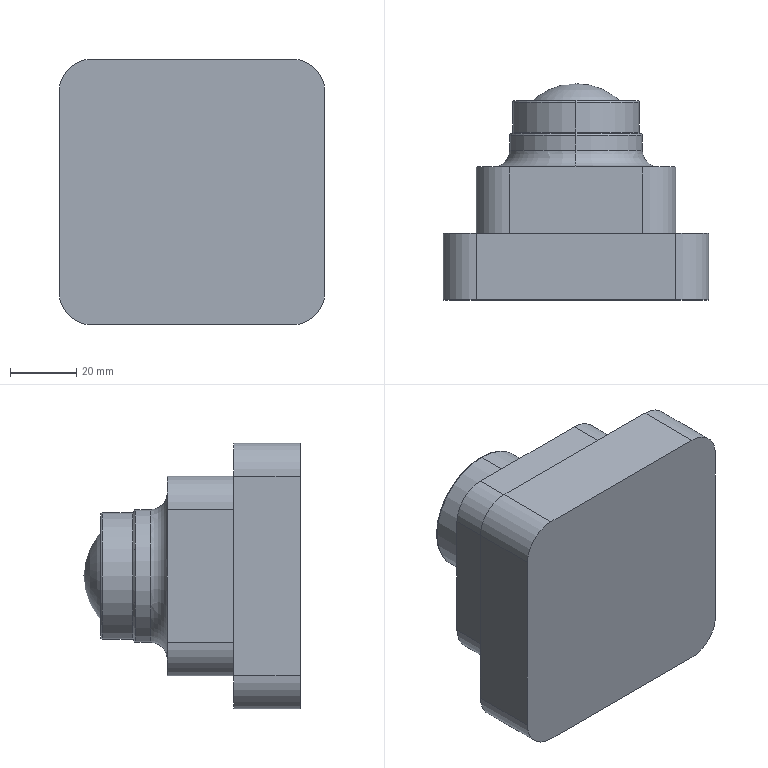Part | SolidWorks | features ICE 5, Fillet 2, Dome 1, Extrusion 1 | 1 solid | 40 faces | box 80 x 65.1 x 80 mm | volume 221973 mm3 | cylinder 16 | plane 13 | torus 10 | sphere 1 | commonest cylinder face diameters 20 x8 30 x2 35 x2 38 x2 40 x2
STEP:
#1=CARTESIAN_POINT('',(0.,49.5,-20.));
#2=VERTEX_POINT('',#1);
#3=CARTESIAN_POINT('',(0.,49.5,20.));
#4=VERTEX_POINT('',#3);
#5=CARTESIAN_POINT('',(0.,49.5,0.));
#6=DIRECTION('',(0.,-1.,0.));
#7=DIRECTION('',(0.,0.,1.));
#8=AXIS2_PLACEMENT_3D('',#5,#6,#7);
#9=CIRCLE('',#8,20.);
#10=EDGE_CURVE('',#2,#4,#9,.T.);
#11=ORIENTED_EDGE('',*,*,#10,.F.);
#12=CARTESIAN_POINT('',(0.,50.,-19.5));
#13=VERTEX_POINT('',#12);
#14=CARTESIAN_POINT('',(0.,49.5,-19.5));
#15=DIRECTION('',(1.,0.,0.));
#16=DIRECTION('',(0.,0.,-1.));
#17=AXIS2_PLACEMENT_3D('',#14,#15,#16);
#18=CIRCLE('',#17,0.5);
#19=EDGE_CURVE('',#2,#13,#18,.T.);
#20=ORIENTED_EDGE('',*,*,#19,.T.);
#21=CARTESIAN_POINT('',(0.,50.,19.5));
#22=VERTEX_POINT('',#21);
#23=CARTESIAN_POINT('',(0.,50.,0.));
#24=DIRECTION('',(0.,-1.,0.));
#25=DIRECTION('',(0.,0.,1.));
#26=AXIS2_PLACEMENT_3D('',#23,#24,#25);
#27=CIRCLE('',#26,19.5);
#28=EDGE_CURVE('',#13,#22,#27,.T.);
#29=ORIENTED_EDGE('',*,*,#28,.T.);
#30=CARTESIAN_POINT('',(0.,49.5,19.5));
#31=DIRECTION('',(-1.,0.,0.));
#32=DIRECTION('',(0.,0.,1.));
#33=AXIS2_PLACEMENT_3D('',#30,#31,#32);
#34=CIRCLE('',#33,0.5);
#35=EDGE_CURVE('',#4,#22,#34,.T.);
#36=ORIENTED_EDGE('',*,*,#35,.F.);
#37=EDGE_LOOP('',(#11,#20,#29,#36));
#38=FACE_OUTER_BOUND('',#37,.T.);
#39=CARTESIAN_POINT('',(0.,49.5,0.));
#40=DIRECTION('',(0.,1.,0.));
#41=DIRECTION('',(0.,0.,1.));
#42=AXIS2_PLACEMENT_3D('',#39,#40,#41);
#43=TOROIDAL_SURFACE('',#42,19.5,0.5);
#44=ADVANCED_FACE('',(#38),#43,.T.);
#45=CARTESIAN_POINT('',(0.,50.5,-19.));
#46=VERTEX_POINT('',#45);
#47=CARTESIAN_POINT('',(0.,50.5,19.));
#48=VERTEX_POINT('',#47);
#49=CARTESIAN_POINT('',(0.,50.5,0.));
#50=DIRECTION('',(0.,1.,0.));
#51=DIRECTION('',(0.,0.,1.));
#52=AXIS2_PLACEMENT_3D('',#49,#50,#51);
#53=CIRCLE('',#52,19.);
#54=EDGE_CURVE('',#46,#48,#53,.T.);
#55=ORIENTED_EDGE('',*,*,#54,.F.);
#56=CARTESIAN_POINT('',(0.,50.5,-19.5));
#57=DIRECTION('',(1.,0.,0.));
#58=DIRECTION('',(0.,0.,-1.));
#59=AXIS2_PLACEMENT_3D('',#56,#57,#58);
#60=CIRCLE('',#59,0.5);
#61=EDGE_CURVE('',#46,#13,#60,.T.);
#62=ORIENTED_EDGE('',*,*,#61,.T.);
#63=CARTESIAN_POINT('',(0.,50.,0.));
#64=DIRECTION('',(0.,-1.,0.));
#65=DIRECTION('',(0.,0.,1.));
#66=AXIS2_PLACEMENT_3D('',#63,#64,#65);
#67=CIRCLE('',#66,19.5);
#68=EDGE_CURVE('',#22,#13,#67,.T.);
#69=ORIENTED_EDGE('',*,*,#68,.F.);
#70=CARTESIAN_POINT('',(0.,50.5,19.5));
#71=DIRECTION('',(-1.,0.,0.));
#72=DIRECTION('',(0.,0.,1.));
#73=AXIS2_PLACEMENT_3D('',#70,#71,#72);
#74=CIRCLE('',#73,0.5);
#75=EDGE_CURVE('',#48,#22,#74,.T.);
#76=ORIENTED_EDGE('',*,*,#75,.F.);
#77=EDGE_LOOP('',(#55,#62,#69,#76));
#78=FACE_OUTER_BOUND('',#77,.T.);
#79=CARTESIAN_POINT('',(0.,50.5,0.));
#80=DIRECTION('',(0.,1.,0.));
#81=DIRECTION('',(0.,0.,1.));
#82=AXIS2_PLACEMENT_3D('',#79,#80,#81);
#83=TOROIDAL_SURFACE('',#82,19.5,0.5);
#84=ADVANCED_FACE('',(#78),#83,.F.);
#85=CARTESIAN_POINT('',(0.,59.5,-19.));
#86=VERTEX_POINT('',#85);
#87=CARTESIAN_POINT('',(0.,59.5,19.));
#88=VERTEX_POINT('',#87);
#89=CARTESIAN_POINT('',(0.,59.5,0.));
#90=DIRECTION('',(0.,-1.,0.));
#91=DIRECTION('',(0.,0.,1.));
#92=AXIS2_PLACEMENT_3D('',#89,#90,#91);
#93=CIRCLE('',#92,19.);
#94=EDGE_CURVE('',#86,#88,#93,.T.);
#95=ORIENTED_EDGE('',*,*,#94,.F.);
#96=CARTESIAN_POINT('',(0.,60.,-18.5));
#97=VERTEX_POINT('',#96);
#98=CARTESIAN_POINT('',(0.,59.5,-18.5));
#99=DIRECTION('',(1.,0.,0.));
#100=DIRECTION('',(0.,0.,-1.));
#101=AXIS2_PLACEMENT_3D('',#98,#99,#100);
#102=CIRCLE('',#101,0.5);
#103=EDGE_CURVE('',#86,#97,#102,.T.);
#104=ORIENTED_EDGE('',*,*,#103,.T.);
#105=CARTESIAN_POINT('',(0.,60.,18.5));
#106=VERTEX_POINT('',#105);
#107=CARTESIAN_POINT('',(0.,60.,0.));
#108=DIRECTION('',(0.,1.,0.));
#109=DIRECTION('',(0.,0.,1.));
#110=AXIS2_PLACEMENT_3D('',#107,#108,#109);
#111=CIRCLE('',#110,18.5);
#112=EDGE_CURVE('',#106,#97,#111,.T.);
#113=ORIENTED_EDGE('',*,*,#112,.F.);
#114=CARTESIAN_POINT('',(0.,59.5,18.5));
#115=DIRECTION('',(-1.,0.,0.));
#116=DIRECTION('',(0.,0.,1.));
#117=AXIS2_PLACEMENT_3D('',#114,#115,#116);
#118=CIRCLE('',#117,0.5);
#119=EDGE_CURVE('',#88,#106,#118,.T.);
#120=ORIENTED_EDGE('',*,*,#119,.F.);
#121=EDGE_LOOP('',(#95,#104,#113,#120));
#122=FACE_OUTER_BOUND('',#121,.T.);
#123=CARTESIAN_POINT('',(0.,59.5,0.));
#124=DIRECTION('',(0.,1.,0.));
#125=DIRECTION('',(0.,0.,1.));
#126=AXIS2_PLACEMENT_3D('',#123,#124,#125);
#127=TOROIDAL_SURFACE('',#126,18.5,0.5);
#128=ADVANCED_FACE('',(#122),#127,.T.);
#129=CARTESIAN_POINT('',(0.,60.,-18.));
#130=VERTEX_POINT('',#129);
#131=CARTESIAN_POINT('',(0.,60.,18.));
#132=VERTEX_POINT('',#131);
#133=CARTESIAN_POINT('',(0.,60.,0.));
#134=DIRECTION('',(0.,-1.,0.));
#135=DIRECTION('',(0.,0.,1.));
#136=AXIS2_PLACEMENT_3D('',#133,#134,#135);
#137=CIRCLE('',#136,18.);
#138=EDGE_CURVE('',#130,#132,#137,.T.);
#139=ORIENTED_EDGE('',*,*,#138,.F.);
#140=CARTESIAN_POINT('',(0.,59.5,-17.5));
#141=VERTEX_POINT('',#140);
#142=CARTESIAN_POINT('',(0.,59.5,-18.));
#143=DIRECTION('',(1.,0.,0.));
#144=DIRECTION('',(0.,0.,-1.));
#145=AXIS2_PLACEMENT_3D('',#142,#143,#144);
#146=CIRCLE('',#145,0.5);
#147=EDGE_CURVE('',#130,#141,#146,.T.);
#148=ORIENTED_EDGE('',*,*,#147,.T.);
#149=CARTESIAN_POINT('',(0.,59.5,17.5));
#150=VERTEX_POINT('',#149);
#151=CARTESIAN_POINT('',(0.,59.5,0.));
#152=DIRECTION('',(0.,1.,0.));
#153=DIRECTION('',(0.,0.,1.));
#154=AXIS2_PLACEMENT_3D('',#151,#152,#153);
#155=CIRCLE('',#154,17.5);
#156=EDGE_CURVE('',#150,#141,#155,.T.);
#157=ORIENTED_EDGE('',*,*,#156,.F.);
#158=CARTESIAN_POINT('',(0.,59.5,18.));
#159=DIRECTION('',(-1.,0.,0.));
#160=DIRECTION('',(0.,0.,1.));
#161=AXIS2_PLACEMENT_3D('',#158,#159,#160);
#162=CIRCLE('',#161,0.5);
#163=EDGE_CURVE('',#132,#150,#162,.T.);
#164=ORIENTED_EDGE('',*,*,#163,.F.);
#165=EDGE_LOOP('',(#139,#148,#157,#164));
#166=FACE_OUTER_BOUND('',#165,.T.);
#167=CARTESIAN_POINT('',(0.,59.5,0.));
#168=DIRECTION('',(0.,1.,0.));
#169=DIRECTION('',(0.,0.,1.));
#170=AXIS2_PLACEMENT_3D('',#167,#168,#169);
#171=TOROIDAL_SURFACE('',#170,18.,0.5);
#172=ADVANCED_FACE('',(#166),#171,.T.);
#173=CARTESIAN_POINT('',(0.,40.,25.));
#174=VERTEX_POINT('',#173);
#175=CARTESIAN_POINT('',(0.,40.,-25.));
#176=VERTEX_POINT('',#175);
#177=CARTESIAN_POINT('',(0.,40.,0.));
#178=DIRECTION('',(0.,-1.,0.));
#179=DIRECTION('',(0.,0.,-1.));
#180=AXIS2_PLACEMENT_3D('',#177,#178,#179);
#181=CIRCLE('',#180,25.);
#182=EDGE_CURVE('',#174,#176,#181,.T.);
#183=ORIENTED_EDGE('',*,*,#182,.F.);
#184=CARTESIAN_POINT('',(0.,45.,20.));
#185=VERTEX_POINT('',#184);
#186=CARTESIAN_POINT('',(0.,45.,25.));
#187=DIRECTION('',(1.,0.,0.));
#188=DIRECTION('',(0.,0.,-1.));
#189=AXIS2_PLACEMENT_3D('',#186,#187,#188);
#190=CIRCLE('',#189,5.);
#191=EDGE_CURVE('',#174,#185,#190,.T.);
#192=ORIENTED_EDGE('',*,*,#191,.T.);
#193=CARTESIAN_POINT('',(0.,45.,-20.));
#194=VERTEX_POINT('',#193);
#195=CARTESIAN_POINT('',(0.,45.,0.));
#196=DIRECTION('',(0.,1.,0.));
#197=DIRECTION('',(0.,0.,-1.));
#198=AXIS2_PLACEMENT_3D('',#195,#196,#197);
#199=CIRCLE('',#198,20.);
#200=EDGE_CURVE('',#194,#185,#199,.T.);
#201=ORIENTED_EDGE('',*,*,#200,.F.);
#202=CARTESIAN_POINT('',(0.,45.,-25.));
#203=DIRECTION('',(-1.,0.,0.));
#204=DIRECTION('',(0.,0.,1.));
#205=AXIS2_PLACEMENT_3D('',#202,#203,#204);
#206=CIRCLE('',#205,5.);
#207=EDGE_CURVE('',#176,#194,#206,.T.);
#208=ORIENTED_EDGE('',*,*,#207,.F.);
#209=EDGE_LOOP('',(#183,#192,#201,#208));
#210=FACE_OUTER_BOUND('',#209,.T.);
#211=CARTESIAN_POINT('',(0.,45.,0.));
#212=DIRECTION('',(0.,-1.,0.));
#213=DIRECTION('',(0.,0.,-1.));
#214=AXIS2_PLACEMENT_3D('',#211,#212,#213);
#215=TOROIDAL_SURFACE('',#214,25.,5.);
#216=ADVANCED_FACE('',(#210),#215,.F.);
#217=CARTESIAN_POINT('',(0.,58.1,15.));
#218=VERTEX_POINT('',#217);
#219=CARTESIAN_POINT('',(0.,58.1,-15.));
#220=VERTEX_POINT('',#219);
#221=CARTESIAN_POINT('',(0.,58.1,0.));
#222=DIRECTION('',(0.,1.,0.));
#223=DIRECTION('',(0.,0.,1.));
#224=AXIS2_PLACEMENT_3D('',#221,#222,#223);
#225=CIRCLE('',#224,15.);
#226=EDGE_CURVE('',#218,#220,#225,.T.);
#227=ORIENTED_EDGE('',*,*,#226,.F.);
#228=CARTESIAN_POINT('',(0.,58.,15.));
#229=VERTEX_POINT('',#228);
#230=CARTESIAN_POINT('',(0.,58.1,15.));
#231=DIRECTION('',(0.,-1.,0.));
#232=VECTOR('',#231,1000.);
#233=LINE('',#230,#232);
#234=EDGE_CURVE('',#218,#229,#233,.T.);
#235=ORIENTED_EDGE('',*,*,#234,.T.);
#236=CARTESIAN_POINT('',(0.,58.,-15.));
#237=VERTEX_POINT('',#236);
#238=CARTESIAN_POINT('',(0.,58.,0.));
#239=DIRECTION('',(0.,1.,0.));
#240=DIRECTION('',(0.,0.,1.));
#241=AXIS2_PLACEMENT_3D('',#238,#239,#240);
#242=CIRCLE('',#241,15.);
#243=EDGE_CURVE('',#229,#237,#242,.T.);
#244=ORIENTED_EDGE('',*,*,#243,.T.);
#245=CARTESIAN_POINT('',(0.,58.1,-15.));
#246=DIRECTION('',(0.,-1.,0.));
#247=VECTOR('',#246,1000.);
#248=LINE('',#245,#247);
#249=EDGE_CURVE('',#220,#237,#248,.T.);
#250=ORIENTED_EDGE('',*,*,#249,.F.);
#251=EDGE_LOOP('',(#227,#235,#244,#250));
#252=FACE_OUTER_BOUND('',#251,.T.);
#253=CARTESIAN_POINT('',(0.,58.1,0.));
#254=DIRECTION('',(0.,-1.,0.));
#255=DIRECTION('',(0.,0.,-1.));
#256=AXIS2_PLACEMENT_3D('',#253,#254,#255);
#257=CYLINDRICAL_SURFACE('',#256,15.);
#258=ADVANCED_FACE('',(#252),#257,.T.);
#259=CARTESIAN_POINT('',(0.,58.,-17.5));
#260=VERTEX_POINT('',#259);
#261=CARTESIAN_POINT('',(0.,58.,17.5));
#262=VERTEX_POINT('',#261);
#263=CARTESIAN_POINT('',(0.,58.,0.));
#264=DIRECTION('',(0.,1.,0.));
#265=DIRECTION('',(0.,0.,1.));
#266=AXIS2_PLACEMENT_3D('',#263,#264,#265);
#267=CIRCLE('',#266,17.5);
#268=EDGE_CURVE('',#260,#262,#267,.T.);
#269=ORIENTED_EDGE('',*,*,#268,.F.);
#270=CARTESIAN_POINT('',(0.,58.,-17.5));
#271=DIRECTION('',(0.,1.,0.));
#272=VECTOR('',#271,1000.);
#273=LINE('',#270,#272);
#274=EDGE_CURVE('',#260,#141,#273,.T.);
#275=ORIENTED_EDGE('',*,*,#274,.T.);
#276=CARTESIAN_POINT('',(0.,59.5,0.));
#277=DIRECTION('',(0.,1.,0.));
#278=DIRECTION('',(0.,0.,1.));
#279=AXIS2_PLACEMENT_3D('',#276,#277,#278);
#280=CIRCLE('',#279,17.5);
#281=EDGE_CURVE('',#141,#150,#280,.T.);
#282=ORIENTED_EDGE('',*,*,#281,.T.);
#283=CARTESIAN_POINT('',(0.,58.,17.5));
#284=DIRECTION('',(0.,1.,0.));
#285=VECTOR('',#284,1000.);
#286=LINE('',#283,#285);
#287=EDGE_CURVE('',#262,#150,#286,.T.);
#288=ORIENTED_EDGE('',*,*,#287,.F.);
#289=EDGE_LOOP('',(#269,#275,#282,#288));
#290=FACE_OUTER_BOUND('',#289,.T.);
#291=CARTESIAN_POINT('',(0.,58.,0.));
#292=DIRECTION('',(0.,1.,0.));
#293=DIRECTION('',(0.,0.,1.));
#294=AXIS2_PLACEMENT_3D('',#291,#292,#293);
#295=CYLINDRICAL_SURFACE('',#294,17.5);
#296=ADVANCED_FACE('',(#290),#295,.F.);
#297=ORIENTED_EDGE('',*,*,#94,.T.);
#298=CARTESIAN_POINT('',(0.,60.,19.));
#299=DIRECTION('',(0.,-1.,0.));
#300=VECTOR('',#299,1000.);
#301=LINE('',#298,#300);
#302=EDGE_CURVE('',#88,#48,#301,.T.);
#303=ORIENTED_EDGE('',*,*,#302,.T.);
#304=CARTESIAN_POINT('',(0.,50.5,0.));
#305=DIRECTION('',(0.,1.,0.));
#306=DIRECTION('',(0.,0.,1.));
#307=AXIS2_PLACEMENT_3D('',#304,#305,#306);
#308=CIRCLE('',#307,19.);
#309=EDGE_CURVE('',#48,#46,#308,.T.);
#310=ORIENTED_EDGE('',*,*,#309,.T.);
#311=CARTESIAN_POINT('',(0.,60.,-19.));
#312=DIRECTION('',(0.,-1.,0.));
#313=VECTOR('',#312,1000.);
#314=LINE('',#311,#313);
#315=EDGE_CURVE('',#86,#46,#314,.T.);
#316=ORIENTED_EDGE('',*,*,#315,.F.);
#317=EDGE_LOOP('',(#297,#303,#310,#316));
#318=FACE_OUTER_BOUND('',#317,.T.);
#319=CARTESIAN_POINT('',(0.,60.,0.));
#320=DIRECTION('',(0.,-1.,0.));
#321=DIRECTION('',(0.,0.,-1.));
#322=AXIS2_PLACEMENT_3D('',#319,#320,#321);
#323=CYLINDRICAL_SURFACE('',#322,19.);
#324=ADVANCED_FACE('',(#318),#323,.T.);
#325=ORIENTED_EDGE('',*,*,#10,.T.);
#326=CARTESIAN_POINT('',(0.,50.,20.));
#327=DIRECTION('',(0.,-1.,0.));
#328=VECTOR('',#327,1000.);
#329=LINE('',#326,#328);
#330=EDGE_CURVE('',#4,#185,#329,.T.);
#331=ORIENTED_EDGE('',*,*,#330,.T.);
#332=CARTESIAN_POINT('',(0.,45.,0.));
#333=DIRECTION('',(0.,1.,0.));
#334=DIRECTION('',(0.,0.,-1.));
#335=AXIS2_PLACEMENT_3D('',#332,#333,#334);
#336=CIRCLE('',#335,20.);
#337=EDGE_CURVE('',#185,#194,#336,.T.);
#338=ORIENTED_EDGE('',*,*,#337,.T.);
#339=CARTESIAN_POINT('',(0.,50.,-20.));
#340=DIRECTION('',(0.,-1.,0.));
#341=VECTOR('',#340,1000.);
#342=LINE('',#339,#341);
#343=EDGE_CURVE('',#2,#194,#342,.T.);
#344=ORIENTED_EDGE('',*,*,#343,.F.);
#345=EDGE_LOOP('',(#325,#331,#338,#344));
#346=FACE_OUTER_BOUND('',#345,.T.);
#347=CARTESIAN_POINT('',(0.,50.,0.));
#348=DIRECTION('',(0.,-1.,0.));
#349=DIRECTION('',(0.,0.,-1.));
#350=AXIS2_PLACEMENT_3D('',#347,#348,#349);
#351=CYLINDRICAL_SURFACE('',#350,20.);
#352=ADVANCED_FACE('',(#346),#351,.T.);
#353=CARTESIAN_POINT('',(-40.,20.,30.));
#354=VERTEX_POINT('',#353);
#355=CARTESIAN_POINT('',(-30.,20.,40.));
#356=VERTEX_POINT('',#355);
#357=CARTESIAN_POINT('',(-30.,20.,30.));
#358=DIRECTION('',(0.,1.,0.));
#359=DIRECTION('',(0.,0.,-1.));
#360=AXIS2_PLACEMENT_3D('',#357,#358,#359);
#361=CIRCLE('',#360,10.);
#362=EDGE_CURVE('',#354,#356,#361,.T.);
#363=ORIENTED_EDGE('',*,*,#362,.T.);
#364=CARTESIAN_POINT('',(30.,20.,40.));
#365=VERTEX_POINT('',#364);
#366=CARTESIAN_POINT('',(-30.,20.,40.));
#367=DIRECTION('',(1.,0.,0.));
#368=VECTOR('',#367,1000.);
#369=LINE('',#366,#368);
#370=EDGE_CURVE('',#356,#365,#369,.T.);
#371=ORIENTED_EDGE('',*,*,#370,.T.);
#372=CARTESIAN_POINT('',(40.,20.,30.));
#373=VERTEX_POINT('',#372);
#374=CARTESIAN_POINT('',(30.,20.,30.));
#375=DIRECTION('',(0.,1.,0.));
#376=DIRECTION('',(0.,0.,1.));
#377=AXIS2_PLACEMENT_3D('',#374,#375,#376);
#378=CIRCLE('',#377,10.);
#379=EDGE_CURVE('',#365,#373,#378,.T.);
#380=ORIENTED_EDGE('',*,*,#379,.T.);
#381=CARTESIAN_POINT('',(40.,20.,-30.));
#382=VERTEX_POINT('',#381);
#383=CARTESIAN_POINT('',(40.,20.,30.));
#384=DIRECTION('',(0.,0.,-1.));
#385=VECTOR('',#384,1000.);
#386=LINE('',#383,#385);
#387=EDGE_CURVE('',#373,#382,#386,.T.);
#388=ORIENTED_EDGE('',*,*,#387,.T.);
#389=CARTESIAN_POINT('',(30.,20.,-40.));
#390=VERTEX_POINT('',#389);
#391=CARTESIAN_POINT('',(30.,20.,-30.));
#392=DIRECTION('',(0.,1.,0.));
#393=DIRECTION('',(0.,0.,-1.));
#394=AXIS2_PLACEMENT_3D('',#391,#392,#393);
#395=CIRCLE('',#394,10.);
#396=EDGE_CURVE('',#382,#390,#395,.T.);
#397=ORIENTED_EDGE('',*,*,#396,.T.);
#398=CARTESIAN_POINT('',(-30.,20.,-40.));
#399=VERTEX_POINT('',#398);
#400=CARTESIAN_POINT('',(-30.,20.,-40.));
#401=DIRECTION('',(-1.,0.,0.));
#402=VECTOR('',#401,1000.);
#403=LINE('',#400,#402);
#404=EDGE_CURVE('',#390,#399,#403,.T.);
#405=ORIENTED_EDGE('',*,*,#404,.T.);
#406=CARTESIAN_POINT('',(-40.,20.,-30.));
#407=VERTEX_POINT('',#406);
#408=CARTESIAN_POINT('',(-30.,20.,-30.));
#409=DIRECTION('',(0.,1.,0.));
#410=DIRECTION('',(0.,0.,-1.));
#411=AXIS2_PLACEMENT_3D('',#408,#409,#410);
#412=CIRCLE('',#411,10.);
#413=EDGE_CURVE('',#399,#407,#412,.T.);
#414=ORIENTED_EDGE('',*,*,#413,.T.);
#415=CARTESIAN_POINT('',(-40.,20.,30.));
#416=DIRECTION('',(0.,0.,1.));
#417=VECTOR('',#416,1000.);
#418=LINE('',#415,#417);
#419=EDGE_CURVE('',#407,#354,#418,.T.);
#420=ORIENTED_EDGE('',*,*,#419,.T.);
#421=EDGE_LOOP('',(#363,#371,#380,#388,#397,#405,#414,#420));
#422=FACE_OUTER_BOUND('',#421,.T.);
#423=CARTESIAN_POINT('',(-30.,20.,20.));
#424=VERTEX_POINT('',#423);
#425=CARTESIAN_POINT('',(-20.,20.,30.));
#426=VERTEX_POINT('',#425);
#427=CARTESIAN_POINT('',(-20.,20.,20.));
#428=DIRECTION('',(0.,1.,0.));
#429=DIRECTION('',(0.,0.,-1.));
#430=AXIS2_PLACEMENT_3D('',#427,#428,#429);
#431=CIRCLE('',#430,10.);
#432=EDGE_CURVE('',#424,#426,#431,.T.);
#433=ORIENTED_EDGE('',*,*,#432,.F.);
#434=CARTESIAN_POINT('',(-30.,20.,-20.));
#435=VERTEX_POINT('',#434);
#436=CARTESIAN_POINT('',(-30.,20.,20.));
#437=DIRECTION('',(0.,0.,1.));
#438=VECTOR('',#437,1000.);
#439=LINE('',#436,#438);
#440=EDGE_CURVE('',#435,#424,#439,.T.);
#441=ORIENTED_EDGE('',*,*,#440,.F.);
#442=CARTESIAN_POINT('',(-20.,20.,-30.));
#443=VERTEX_POINT('',#442);
#444=CARTESIAN_POINT('',(-20.,20.,-20.));
#445=DIRECTION('',(0.,1.,0.));
#446=DIRECTION('',(0.,0.,-1.));
#447=AXIS2_PLACEMENT_3D('',#444,#445,#446);
#448=CIRCLE('',#447,10.);
#449=EDGE_CURVE('',#443,#435,#448,.T.);
#450=ORIENTED_EDGE('',*,*,#449,.F.);
#451=CARTESIAN_POINT('',(20.,20.,-30.));
#452=VERTEX_POINT('',#451);
#453=CARTESIAN_POINT('',(-20.,20.,-30.));
#454=DIRECTION('',(-1.,0.,0.));
#455=VECTOR('',#454,1000.);
#456=LINE('',#453,#455);
#457=EDGE_CURVE('',#452,#443,#456,.T.);
#458=ORIENTED_EDGE('',*,*,#457,.F.);
#459=CARTESIAN_POINT('',(30.,20.,-20.));
#460=VERTEX_POINT('',#459);
#461=CARTESIAN_POINT('',(20.,20.,-20.));
#462=DIRECTION('',(0.,1.,0.));
#463=DIRECTION('',(0.,0.,-1.));
#464=AXIS2_PLACEMENT_3D('',#461,#462,#463);
#465=CIRCLE('',#464,10.);
#466=EDGE_CURVE('',#460,#452,#465,.T.);
#467=ORIENTED_EDGE('',*,*,#466,.F.);
#468=CARTESIAN_POINT('',(30.,20.,20.));
#469=VERTEX_POINT('',#468);
#470=CARTESIAN_POINT('',(30.,20.,20.));
#471=DIRECTION('',(0.,0.,-1.));
#472=VECTOR('',#471,1000.);
#473=LINE('',#470,#472);
#474=EDGE_CURVE('',#469,#460,#473,.T.);
#475=ORIENTED_EDGE('',*,*,#474,.F.);
#476=CARTESIAN_POINT('',(20.,20.,30.));
#477=VERTEX_POINT('',#476);
#478=CARTESIAN_POINT('',(20.,20.,20.));
#479=DIRECTION('',(0.,1.,0.));
#480=DIRECTION('',(0.,0.,1.));
#481=AXIS2_PLACEMENT_3D('',#478,#479,#480);
#482=CIRCLE('',#481,10.);
#483=EDGE_CURVE('',#477,#469,#482,.T.);
#484=ORIENTED_EDGE('',*,*,#483,.F.);
#485=CARTESIAN_POINT('',(-20.,20.,30.));
#486=DIRECTION('',(1.,0.,0.));
#487=VECTOR('',#486,1000.);
#488=LINE('',#485,#487);
#489=EDGE_CURVE('',#426,#477,#488,.T.);
#490=ORIENTED_EDGE('',*,*,#489,.F.);
#491=EDGE_LOOP('',(#433,#441,#450,#458,#467,#475,#484,#490));
#492=FACE_BOUND('',#491,.T.);
#493=CARTESIAN_POINT('',(-30.,20.,30.));
#494=DIRECTION('',(0.,-1.,0.));
#495=DIRECTION('',(0.,0.,-1.));
#496=AXIS2_PLACEMENT_3D('',#493,#494,#495);
#497=PLANE('',#496);
#498=ADVANCED_FACE('',(#422,#492),#497,.F.);
#499=CARTESIAN_POINT('',(-40.,0.,30.));
#500=VERTEX_POINT('',#499);
#501=CARTESIAN_POINT('',(-30.,0.,40.));
#502=VERTEX_POINT('',#501);
#503=CARTESIAN_POINT('',(-30.,0.,30.));
#504=DIRECTION('',(0.,1.,0.));
#505=DIRECTION('',(0.,0.,-1.));
#506=AXIS2_PLACEMENT_3D('',#503,#504,#505);
#507=CIRCLE('',#506,10.);
#508=EDGE_CURVE('',#500,#502,#507,.T.);
#509=ORIENTED_EDGE('',*,*,#508,.T.);
#510=CARTESIAN_POINT('',(-30.,20.,40.));
#511=DIRECTION('',(0.,-1.,0.));
#512=VECTOR('',#511,1000.);
#513=LINE('',#510,#512);
#514=EDGE_CURVE('',#356,#502,#513,.T.);
#515=ORIENTED_EDGE('',*,*,#514,.F.);
#516=ORIENTED_EDGE('',*,*,#362,.F.);
#517=CARTESIAN_POINT('',(-40.,20.,30.));
#518=DIRECTION('',(0.,-1.,0.));
#519=VECTOR('',#518,1000.);
#520=LINE('',#517,#519);
#521=EDGE_CURVE('',#354,#500,#520,.T.);
#522=ORIENTED_EDGE('',*,*,#521,.T.);
#523=EDGE_LOOP('',(#509,#515,#516,#522));
#524=FACE_OUTER_BOUND('',#523,.T.);
#525=CARTESIAN_POINT('',(-30.,20.,30.));
#526=DIRECTION('',(0.,-1.,0.));
#527=DIRECTION('',(0.,0.,-1.));
#528=AXIS2_PLACEMENT_3D('',#525,#526,#527);
#529=CYLINDRICAL_SURFACE('',#528,10.);
#530=ADVANCED_FACE('',(#524),#529,.T.);
#531=CARTESIAN_POINT('',(30.,0.,40.));
#532=VERTEX_POINT('',#531);
#533=CARTESIAN_POINT('',(-30.,0.,40.));
#534=DIRECTION('',(1.,0.,0.));
#535=VECTOR('',#534,1000.);
#536=LINE('',#533,#535);
#537=EDGE_CURVE('',#502,#532,#536,.T.);
#538=ORIENTED_EDGE('',*,*,#537,.T.);
#539=CARTESIAN_POINT('',(30.,20.,40.));
#540=DIRECTION('',(0.,-1.,0.));
#541=VECTOR('',#540,1000.);
#542=LINE('',#539,#541);
#543=EDGE_CURVE('',#365,#532,#542,.T.);
#544=ORIENTED_EDGE('',*,*,#543,.F.);
#545=ORIENTED_EDGE('',*,*,#370,.F.);
#546=ORIENTED_EDGE('',*,*,#514,.T.);
#547=EDGE_LOOP('',(#538,#544,#545,#546));
#548=FACE_OUTER_BOUND('',#547,.T.);
#549=CARTESIAN_POINT('',(-30.,20.,40.));
#550=DIRECTION('',(0.,0.,-1.));
#551=DIRECTION('',(-1.,0.,0.));
#552=AXIS2_PLACEMENT_3D('',#549,#550,#551);
#553=PLANE('',#552);
#554=ADVANCED_FACE('',(#548),#553,.F.);
#555=CARTESIAN_POINT('',(40.,0.,30.));
#556=VERTEX_POINT('',#555);
#557=CARTESIAN_POINT('',(30.,0.,30.));
#558=DIRECTION('',(0.,1.,0.));
#559=DIRECTION('',(0.,0.,1.));
#560=AXIS2_PLACEMENT_3D('',#557,#558,#559);
#561=CIRCLE('',#560,10.);
#562=EDGE_CURVE('',#532,#556,#561,.T.);
#563=ORIENTED_EDGE('',*,*,#562,.T.);
#564=CARTESIAN_POINT('',(40.,20.,30.));
#565=DIRECTION('',(0.,-1.,0.));
#566=VECTOR('',#565,1000.);
#567=LINE('',#564,#566);
#568=EDGE_CURVE('',#373,#556,#567,.T.);
#569=ORIENTED_EDGE('',*,*,#568,.F.);
#570=ORIENTED_EDGE('',*,*,#379,.F.);
#571=ORIENTED_EDGE('',*,*,#543,.T.);
#572=EDGE_LOOP('',(#563,#569,#570,#571));
#573=FACE_OUTER_BOUND('',#572,.T.);
#574=CARTESIAN_POINT('',(30.,20.,30.));
#575=DIRECTION('',(0.,-1.,0.));
#576=DIRECTION('',(0.,0.,-1.));
#577=AXIS2_PLACEMENT_3D('',#574,#575,#576);
#578=CYLINDRICAL_SURFACE('',#577,10.);
#579=ADVANCED_FACE('',(#573),#578,.T.);
#580=CARTESIAN_POINT('',(40.,0.,-30.));
#581=VERTEX_POINT('',#580);
#582=CARTESIAN_POINT('',(40.,0.,30.));
#583=DIRECTION('',(0.,0.,-1.));
#584=VECTOR('',#583,1000.);
#585=LINE('',#582,#584);
#586=EDGE_CURVE('',#556,#581,#585,.T.);
#587=ORIENTED_EDGE('',*,*,#586,.T.);
#588=CARTESIAN_POINT('',(40.,20.,-30.));
#589=DIRECTION('',(0.,-1.,0.));
#590=VECTOR('',#589,1000.);
#591=LINE('',#588,#590);
#592=EDGE_CURVE('',#382,#581,#591,.T.);
#593=ORIENTED_EDGE('',*,*,#592,.F.);
#594=ORIENTED_EDGE('',*,*,#387,.F.);
#595=ORIENTED_EDGE('',*,*,#568,.T.);
#596=EDGE_LOOP('',(#587,#593,#594,#595));
#597=FACE_OUTER_BOUND('',#596,.T.);
#598=CARTESIAN_POINT('',(40.,20.,30.));
#599=DIRECTION('',(-1.,0.,0.));
#600=DIRECTION('',(0.,0.,1.));
#601=AXIS2_PLACEMENT_3D('',#598,#599,#600);
#602=PLANE('',#601);
#603=ADVANCED_FACE('',(#597),#602,.F.);
#604=CARTESIAN_POINT('',(30.,0.,-40.));
#605=VERTEX_POINT('',#604);
#606=CARTESIAN_POINT('',(30.,0.,-30.));
#607=DIRECTION('',(0.,1.,0.));
#608=DIRECTION('',(0.,0.,-1.));
#609=AXIS2_PLACEMENT_3D('',#606,#607,#608);
#610=CIRCLE('',#609,10.);
#611=EDGE_CURVE('',#581,#605,#610,.T.);
#612=ORIENTED_EDGE('',*,*,#611,.T.);
#613=CARTESIAN_POINT('',(30.,20.,-40.));
#614=DIRECTION('',(0.,-1.,0.));
#615=VECTOR('',#614,1000.);
#616=LINE('',#613,#615);
#617=EDGE_CURVE('',#390,#605,#616,.T.);
#618=ORIENTED_EDGE('',*,*,#617,.F.);
#619=ORIENTED_EDGE('',*,*,#396,.F.);
#620=ORIENTED_EDGE('',*,*,#592,.T.);
#621=EDGE_LOOP('',(#612,#618,#619,#620));
#622=FACE_OUTER_BOUND('',#621,.T.);
#623=CARTESIAN_POINT('',(30.,20.,-30.));
#624=DIRECTION('',(0.,-1.,0.));
#625=DIRECTION('',(0.,0.,-1.));
#626=AXIS2_PLACEMENT_3D('',#623,#624,#625);
#627=CYLINDRICAL_SURFACE('',#626,10.);
#628=ADVANCED_FACE('',(#622),#627,.T.);
#629=CARTESIAN_POINT('',(-30.,0.,-40.));
#630=VERTEX_POINT('',#629);
#631=CARTESIAN_POINT('',(-30.,0.,-40.));
#632=DIRECTION('',(-1.,0.,0.));
#633=VECTOR('',#632,1000.);
#634=LINE('',#631,#633);
#635=EDGE_CURVE('',#605,#630,#634,.T.);
#636=ORIENTED_EDGE('',*,*,#635,.T.);
#637=CARTESIAN_POINT('',(-30.,20.,-40.));
#638=DIRECTION('',(0.,-1.,0.));
#639=VECTOR('',#638,1000.);
#640=LINE('',#637,#639);
#641=EDGE_CURVE('',#399,#630,#640,.T.);
#642=ORIENTED_EDGE('',*,*,#641,.F.);
#643=ORIENTED_EDGE('',*,*,#404,.F.);
#644=ORIENTED_EDGE('',*,*,#617,.T.);
#645=EDGE_LOOP('',(#636,#642,#643,#644));
#646=FACE_OUTER_BOUND('',#645,.T.);
#647=CARTESIAN_POINT('',(-30.,20.,-40.));
#648=DIRECTION('',(0.,0.,1.));
#649=DIRECTION('',(1.,0.,0.));
#650=AXIS2_PLACEMENT_3D('',#647,#648,#649);
#651=PLANE('',#650);
#652=ADVANCED_FACE('',(#646),#651,.F.);
#653=CARTESIAN_POINT('',(-40.,0.,-30.));
#654=VERTEX_POINT('',#653);
#655=CARTESIAN_POINT('',(-30.,0.,-30.));
#656=DIRECTION('',(0.,1.,0.));
#657=DIRECTION('',(0.,0.,-1.));
#658=AXIS2_PLACEMENT_3D('',#655,#656,#657);
#659=CIRCLE('',#658,10.);
#660=EDGE_CURVE('',#630,#654,#659,.T.);
#661=ORIENTED_EDGE('',*,*,#660,.T.);
#662=CARTESIAN_POINT('',(-40.,20.,-30.));
#663=DIRECTION('',(0.,-1.,0.));
#664=VECTOR('',#663,1000.);
#665=LINE('',#662,#664);
#666=EDGE_CURVE('',#407,#654,#665,.T.);
#667=ORIENTED_EDGE('',*,*,#666,.F.);
#668=ORIENTED_EDGE('',*,*,#413,.F.);
#669=ORIENTED_EDGE('',*,*,#641,.T.);
#670=EDGE_LOOP('',(#661,#667,#668,#669));
#671=FACE_OUTER_BOUND('',#670,.T.);
#672=CARTESIAN_POINT('',(-30.,20.,-30.));
#673=DIRECTION('',(0.,-1.,0.));
#674=DIRECTION('',(0.,0.,-1.));
#675=AXIS2_PLACEMENT_3D('',#672,#673,#674);
#676=CYLINDRICAL_SURFACE('',#675,10.);
#677=ADVANCED_FACE('',(#671),#676,.T.);
#678=CARTESIAN_POINT('',(-40.,0.,30.));
#679=DIRECTION('',(0.,0.,1.));
#680=VECTOR('',#679,1000.);
#681=LINE('',#678,#680);
#682=EDGE_CURVE('',#654,#500,#681,.T.);
#683=ORIENTED_EDGE('',*,*,#682,.T.);
#684=ORIENTED_EDGE('',*,*,#521,.F.);
#685=ORIENTED_EDGE('',*,*,#419,.F.);
#686=ORIENTED_EDGE('',*,*,#666,.T.);
#687=EDGE_LOOP('',(#683,#684,#685,#686));
#688=FACE_OUTER_BOUND('',#687,.T.);
#689=CARTESIAN_POINT('',(-40.,20.,30.));
#690=DIRECTION('',(1.,0.,0.));
#691=DIRECTION('',(0.,0.,-1.));
#692=AXIS2_PLACEMENT_3D('',#689,#690,#691);
#693=PLANE('',#692);
#694=ADVANCED_FACE('',(#688),#693,.F.);
#695=ORIENTED_EDGE('',*,*,#508,.F.);
#696=ORIENTED_EDGE('',*,*,#682,.F.);
#697=ORIENTED_EDGE('',*,*,#660,.F.);
#698=ORIENTED_EDGE('',*,*,#635,.F.);
#699=ORIENTED_EDGE('',*,*,#611,.F.);
#700=ORIENTED_EDGE('',*,*,#586,.F.);
#701=ORIENTED_EDGE('',*,*,#562,.F.);
#702=ORIENTED_EDGE('',*,*,#537,.F.);
#703=EDGE_LOOP('',(#695,#696,#697,#698,#699,#700,#701,#702));
#704=FACE_OUTER_BOUND('',#703,.T.);
#705=CARTESIAN_POINT('',(-30.,0.,30.));
#706=DIRECTION('',(0.,-1.,0.));
#707=DIRECTION('',(0.,0.,-1.));
#708=AXIS2_PLACEMENT_3D('',#705,#706,#707);
#709=PLANE('',#708);
#710=ADVANCED_FACE('',(#704),#709,.T.);
#711=ORIENTED_EDGE('',*,*,#432,.T.);
#712=CARTESIAN_POINT('',(-20.,40.,30.));
#713=VERTEX_POINT('',#712);
#714=CARTESIAN_POINT('',(-20.,40.,30.));
#715=DIRECTION('',(0.,-1.,0.));
#716=VECTOR('',#715,1000.);
#717=LINE('',#714,#716);
#718=EDGE_CURVE('',#713,#426,#717,.T.);
#719=ORIENTED_EDGE('',*,*,#718,.F.);
#720=CARTESIAN_POINT('',(-30.,40.,20.));
#721=VERTEX_POINT('',#720);
#722=CARTESIAN_POINT('',(-20.,40.,20.));
#723=DIRECTION('',(0.,1.,0.));
#724=DIRECTION('',(0.,0.,-1.));
#725=AXIS2_PLACEMENT_3D('',#722,#723,#724);
#726=CIRCLE('',#725,10.);
#727=EDGE_CURVE('',#721,#713,#726,.T.);
#728=ORIENTED_EDGE('',*,*,#727,.F.);
#729=CARTESIAN_POINT('',(-30.,40.,20.));
#730=DIRECTION('',(0.,-1.,0.));
#731=VECTOR('',#730,1000.);
#732=LINE('',#729,#731);
#733=EDGE_CURVE('',#721,#424,#732,.T.);
#734=ORIENTED_EDGE('',*,*,#733,.T.);
#735=EDGE_LOOP('',(#711,#719,#728,#734));
#736=FACE_OUTER_BOUND('',#735,.T.);
#737=CARTESIAN_POINT('',(-20.,40.,20.));
#738=DIRECTION('',(0.,-1.,0.));
#739=DIRECTION('',(0.,0.,-1.));
#740=AXIS2_PLACEMENT_3D('',#737,#738,#739);
#741=CYLINDRICAL_SURFACE('',#740,10.);
#742=ADVANCED_FACE('',(#736),#741,.T.);
#743=ORIENTED_EDGE('',*,*,#489,.T.);
#744=CARTESIAN_POINT('',(20.,40.,30.));
#745=VERTEX_POINT('',#744);
#746=CARTESIAN_POINT('',(20.,40.,30.));
#747=DIRECTION('',(0.,-1.,0.));
#748=VECTOR('',#747,1000.);
#749=LINE('',#746,#748);
#750=EDGE_CURVE('',#745,#477,#749,.T.);
#751=ORIENTED_EDGE('',*,*,#750,.F.);
#752=CARTESIAN_POINT('',(-20.,40.,30.));
#753=DIRECTION('',(1.,0.,0.));
#754=VECTOR('',#753,1000.);
#755=LINE('',#752,#754);
#756=EDGE_CURVE('',#713,#745,#755,.T.);
#757=ORIENTED_EDGE('',*,*,#756,.F.);
#758=ORIENTED_EDGE('',*,*,#718,.T.);
#759=EDGE_LOOP('',(#743,#751,#757,#758));
#760=FACE_OUTER_BOUND('',#759,.T.);
#761=CARTESIAN_POINT('',(-20.,40.,30.));
#762=DIRECTION('',(0.,0.,-1.));
#763=DIRECTION('',(-1.,0.,0.));
#764=AXIS2_PLACEMENT_3D('',#761,#762,#763);
#765=PLANE('',#764);
#766=ADVANCED_FACE('',(#760),#765,.F.);
#767=ORIENTED_EDGE('',*,*,#483,.T.);
#768=CARTESIAN_POINT('',(30.,40.,20.));
#769=VERTEX_POINT('',#768);
#770=CARTESIAN_POINT('',(30.,40.,20.));
#771=DIRECTION('',(0.,-1.,0.));
#772=VECTOR('',#771,1000.);
#773=LINE('',#770,#772);
#774=EDGE_CURVE('',#769,#469,#773,.T.);
#775=ORIENTED_EDGE('',*,*,#774,.F.);
#776=CARTESIAN_POINT('',(20.,40.,20.));
#777=DIRECTION('',(0.,1.,0.));
#778=DIRECTION('',(0.,0.,1.));
#779=AXIS2_PLACEMENT_3D('',#776,#777,#778);
#780=CIRCLE('',#779,10.);
#781=EDGE_CURVE('',#745,#769,#780,.T.);
#782=ORIENTED_EDGE('',*,*,#781,.F.);
#783=ORIENTED_EDGE('',*,*,#750,.T.);
#784=EDGE_LOOP('',(#767,#775,#782,#783));
#785=FACE_OUTER_BOUND('',#784,.T.);
#786=CARTESIAN_POINT('',(20.,40.,20.));
#787=DIRECTION('',(0.,-1.,0.));
#788=DIRECTION('',(0.,0.,-1.));
#789=AXIS2_PLACEMENT_3D('',#786,#787,#788);
#790=CYLINDRICAL_SURFACE('',#789,10.);
#791=ADVANCED_FACE('',(#785),#790,.T.);
#792=ORIENTED_EDGE('',*,*,#474,.T.);
#793=CARTESIAN_POINT('',(30.,40.,-20.));
#794=VERTEX_POINT('',#793);
#795=CARTESIAN_POINT('',(30.,40.,-20.));
#796=DIRECTION('',(0.,-1.,0.));
#797=VECTOR('',#796,1000.);
#798=LINE('',#795,#797);
#799=EDGE_CURVE('',#794,#460,#798,.T.);
#800=ORIENTED_EDGE('',*,*,#799,.F.);
#801=CARTESIAN_POINT('',(30.,40.,20.));
#802=DIRECTION('',(0.,0.,-1.));
#803=VECTOR('',#802,1000.);
#804=LINE('',#801,#803);
#805=EDGE_CURVE('',#769,#794,#804,.T.);
#806=ORIENTED_EDGE('',*,*,#805,.F.);
#807=ORIENTED_EDGE('',*,*,#774,.T.);
#808=EDGE_LOOP('',(#792,#800,#806,#807));
#809=FACE_OUTER_BOUND('',#808,.T.);
#810=CARTESIAN_POINT('',(30.,40.,20.));
#811=DIRECTION('',(-1.,0.,0.));
#812=DIRECTION('',(0.,0.,1.));
#813=AXIS2_PLACEMENT_3D('',#810,#811,#812);
#814=PLANE('',#813);
#815=ADVANCED_FACE('',(#809),#814,.F.);
#816=ORIENTED_EDGE('',*,*,#466,.T.);
#817=CARTESIAN_POINT('',(20.,40.,-30.));
#818=VERTEX_POINT('',#817);
#819=CARTESIAN_POINT('',(20.,40.,-30.));
#820=DIRECTION('',(0.,-1.,0.));
#821=VECTOR('',#820,1000.);
#822=LINE('',#819,#821);
#823=EDGE_CURVE('',#818,#452,#822,.T.);
#824=ORIENTED_EDGE('',*,*,#823,.F.);
#825=CARTESIAN_POINT('',(20.,40.,-20.));
#826=DIRECTION('',(0.,1.,0.));
#827=DIRECTION('',(0.,0.,-1.));
#828=AXIS2_PLACEMENT_3D('',#825,#826,#827);
#829=CIRCLE('',#828,10.);
#830=EDGE_CURVE('',#794,#818,#829,.T.);
#831=ORIENTED_EDGE('',*,*,#830,.F.);
#832=ORIENTED_EDGE('',*,*,#799,.T.);
#833=EDGE_LOOP('',(#816,#824,#831,#832));
#834=FACE_OUTER_BOUND('',#833,.T.);
#835=CARTESIAN_POINT('',(20.,40.,-20.));
#836=DIRECTION('',(0.,-1.,0.));
#837=DIRECTION('',(0.,0.,-1.));
#838=AXIS2_PLACEMENT_3D('',#835,#836,#837);
#839=CYLINDRICAL_SURFACE('',#838,10.);
#840=ADVANCED_FACE('',(#834),#839,.T.);
#841=ORIENTED_EDGE('',*,*,#457,.T.);
#842=CARTESIAN_POINT('',(-20.,40.,-30.));
#843=VERTEX_POINT('',#842);
#844=CARTESIAN_POINT('',(-20.,40.,-30.));
#845=DIRECTION('',(0.,-1.,0.));
#846=VECTOR('',#845,1000.);
#847=LINE('',#844,#846);
#848=EDGE_CURVE('',#843,#443,#847,.T.);
#849=ORIENTED_EDGE('',*,*,#848,.F.);
#850=CARTESIAN_POINT('',(-20.,40.,-30.));
#851=DIRECTION('',(-1.,0.,0.));
#852=VECTOR('',#851,1000.);
#853=LINE('',#850,#852);
#854=EDGE_CURVE('',#818,#843,#853,.T.);
#855=ORIENTED_EDGE('',*,*,#854,.F.);
#856=ORIENTED_EDGE('',*,*,#823,.T.);
#857=EDGE_LOOP('',(#841,#849,#855,#856));
#858=FACE_OUTER_BOUND('',#857,.T.);
#859=CARTESIAN_POINT('',(-20.,40.,-30.));
#860=DIRECTION('',(0.,0.,1.));
#861=DIRECTION('',(1.,0.,0.));
#862=AXIS2_PLACEMENT_3D('',#859,#860,#861);
#863=PLANE('',#862);
#864=ADVANCED_FACE('',(#858),#863,.F.);
#865=ORIENTED_EDGE('',*,*,#449,.T.);
#866=CARTESIAN_POINT('',(-30.,40.,-20.));
#867=VERTEX_POINT('',#866);
#868=CARTESIAN_POINT('',(-30.,40.,-20.));
#869=DIRECTION('',(0.,-1.,0.));
#870=VECTOR('',#869,1000.);
#871=LINE('',#868,#870);
#872=EDGE_CURVE('',#867,#435,#871,.T.);
#873=ORIENTED_EDGE('',*,*,#872,.F.);
#874=CARTESIAN_POINT('',(-20.,40.,-20.));
#875=DIRECTION('',(0.,1.,0.));
#876=DIRECTION('',(0.,0.,-1.));
#877=AXIS2_PLACEMENT_3D('',#874,#875,#876);
#878=CIRCLE('',#877,10.);
#879=EDGE_CURVE('',#843,#867,#878,.T.);
#880=ORIENTED_EDGE('',*,*,#879,.F.);
#881=ORIENTED_EDGE('',*,*,#848,.T.);
#882=EDGE_LOOP('',(#865,#873,#880,#881));
#883=FACE_OUTER_BOUND('',#882,.T.);
#884=CARTESIAN_POINT('',(-20.,40.,-20.));
#885=DIRECTION('',(0.,-1.,0.));
#886=DIRECTION('',(0.,0.,-1.));
#887=AXIS2_PLACEMENT_3D('',#884,#885,#886);
#888=CYLINDRICAL_SURFACE('',#887,10.);
#889=ADVANCED_FACE('',(#883),#888,.T.);
#890=ORIENTED_EDGE('',*,*,#440,.T.);
#891=ORIENTED_EDGE('',*,*,#733,.F.);
#892=CARTESIAN_POINT('',(-30.,40.,20.));
#893=DIRECTION('',(0.,0.,1.));
#894=VECTOR('',#893,1000.);
#895=LINE('',#892,#894);
#896=EDGE_CURVE('',#867,#721,#895,.T.);
#897=ORIENTED_EDGE('',*,*,#896,.F.);
#898=ORIENTED_EDGE('',*,*,#872,.T.);
#899=EDGE_LOOP('',(#890,#891,#897,#898));
#900=FACE_OUTER_BOUND('',#899,.T.);
#901=CARTESIAN_POINT('',(-30.,40.,20.));
#902=DIRECTION('',(1.,0.,0.));
#903=DIRECTION('',(0.,0.,-1.));
#904=AXIS2_PLACEMENT_3D('',#901,#902,#903);
#905=PLANE('',#904);
#906=ADVANCED_FACE('',(#900),#905,.F.);
#907=CARTESIAN_POINT('',(0.,40.,0.));
#908=DIRECTION('',(0.,-1.,0.));
#909=DIRECTION('',(0.,0.,-1.));
#910=AXIS2_PLACEMENT_3D('',#907,#908,#909);
#911=CIRCLE('',#910,25.);
#912=EDGE_CURVE('',#176,#174,#911,.T.);
#913=ORIENTED_EDGE('',*,*,#912,.T.);
#914=ORIENTED_EDGE('',*,*,#182,.T.);
#915=EDGE_LOOP('',(#913,#914));
#916=FACE_BOUND('',#915,.T.);
#917=ORIENTED_EDGE('',*,*,#727,.T.);
#918=ORIENTED_EDGE('',*,*,#756,.T.);
#919=ORIENTED_EDGE('',*,*,#781,.T.);
#920=ORIENTED_EDGE('',*,*,#805,.T.);
#921=ORIENTED_EDGE('',*,*,#830,.T.);
#922=ORIENTED_EDGE('',*,*,#854,.T.);
#923=ORIENTED_EDGE('',*,*,#879,.T.);
#924=ORIENTED_EDGE('',*,*,#896,.T.);
#925=EDGE_LOOP('',(#917,#918,#919,#920,#921,#922,#923,#924));
#926=FACE_OUTER_BOUND('',#925,.T.);
#927=CARTESIAN_POINT('',(-20.,40.,20.));
#928=DIRECTION('',(0.,-1.,0.));
#929=DIRECTION('',(0.,0.,-1.));
#930=AXIS2_PLACEMENT_3D('',#927,#928,#929);
#931=PLANE('',#930);
#932=ADVANCED_FACE('',(#916,#926),#931,.F.);
#933=ORIENTED_EDGE('',*,*,#330,.F.);
#934=CARTESIAN_POINT('',(0.,49.5,0.));
#935=DIRECTION('',(0.,-1.,0.));
#936=DIRECTION('',(0.,0.,1.));
#937=AXIS2_PLACEMENT_3D('',#934,#935,#936);
#938=CIRCLE('',#937,20.);
#939=EDGE_CURVE('',#4,#2,#938,.T.);
#940=ORIENTED_EDGE('',*,*,#939,.T.);
#941=ORIENTED_EDGE('',*,*,#343,.T.);
#942=ORIENTED_EDGE('',*,*,#200,.T.);
#943=EDGE_LOOP('',(#933,#940,#941,#942));
#944=FACE_OUTER_BOUND('',#943,.T.);
#945=CARTESIAN_POINT('',(0.,50.,0.));
#946=DIRECTION('',(0.,-1.,0.));
#947=DIRECTION('',(0.,0.,-1.));
#948=AXIS2_PLACEMENT_3D('',#945,#946,#947);
#949=CYLINDRICAL_SURFACE('',#948,20.);
#950=ADVANCED_FACE('',(#944),#949,.T.);
#951=ORIENTED_EDGE('',*,*,#302,.F.);
#952=CARTESIAN_POINT('',(0.,59.5,0.));
#953=DIRECTION('',(0.,-1.,0.));
#954=DIRECTION('',(0.,0.,1.));
#955=AXIS2_PLACEMENT_3D('',#952,#953,#954);
#956=CIRCLE('',#955,19.);
#957=EDGE_CURVE('',#88,#86,#956,.T.);
#958=ORIENTED_EDGE('',*,*,#957,.T.);
#959=ORIENTED_EDGE('',*,*,#315,.T.);
#960=ORIENTED_EDGE('',*,*,#54,.T.);
#961=EDGE_LOOP('',(#951,#958,#959,#960));
#962=FACE_OUTER_BOUND('',#961,.T.);
#963=CARTESIAN_POINT('',(0.,60.,0.));
#964=DIRECTION('',(0.,-1.,0.));
#965=DIRECTION('',(0.,0.,-1.));
#966=AXIS2_PLACEMENT_3D('',#963,#964,#965);
#967=CYLINDRICAL_SURFACE('',#966,19.);
#968=ADVANCED_FACE('',(#962),#967,.T.);
#969=CARTESIAN_POINT('',(0.,60.,0.));
#970=DIRECTION('',(0.,-1.,0.));
#971=DIRECTION('',(0.,0.,1.));
#972=AXIS2_PLACEMENT_3D('',#969,#970,#971);
#973=CIRCLE('',#972,18.);
#974=EDGE_CURVE('',#132,#130,#973,.T.);
#975=ORIENTED_EDGE('',*,*,#974,.T.);
#976=ORIENTED_EDGE('',*,*,#138,.T.);
#977=EDGE_LOOP('',(#975,#976));
#978=FACE_BOUND('',#977,.T.);
#979=ORIENTED_EDGE('',*,*,#112,.T.);
#980=CARTESIAN_POINT('',(0.,60.,0.));
#981=DIRECTION('',(0.,1.,0.));
#982=DIRECTION('',(0.,0.,1.));
#983=AXIS2_PLACEMENT_3D('',#980,#981,#982);
#984=CIRCLE('',#983,18.5);
#985=EDGE_CURVE('',#97,#106,#984,.T.);
#986=ORIENTED_EDGE('',*,*,#985,.T.);
#987=EDGE_LOOP('',(#979,#986));
#988=FACE_OUTER_BOUND('',#987,.T.);
#989=CARTESIAN_POINT('',(0.,60.,0.));
#990=DIRECTION('',(0.,1.,0.));
#991=DIRECTION('',(0.,0.,1.));
#992=AXIS2_PLACEMENT_3D('',#989,#990,#991);
#993=PLANE('',#992);
#994=ADVANCED_FACE('',(#978,#988),#993,.T.);
#995=ORIENTED_EDGE('',*,*,#274,.F.);
#996=CARTESIAN_POINT('',(0.,58.,0.));
#997=DIRECTION('',(0.,1.,0.));
#998=DIRECTION('',(0.,0.,1.));
#999=AXIS2_PLACEMENT_3D('',#996,#997,#998);
#1000=CIRCLE('',#999,17.5);
#1001=EDGE_CURVE('',#262,#260,#1000,.T.);
#1002=ORIENTED_EDGE('',*,*,#1001,.F.);
#1003=ORIENTED_EDGE('',*,*,#287,.T.);
#1004=ORIENTED_EDGE('',*,*,#156,.T.);
#1005=EDGE_LOOP('',(#995,#1002,#1003,#1004));
#1006=FACE_OUTER_BOUND('',#1005,.T.);
#1007=CARTESIAN_POINT('',(0.,58.,0.));
#1008=DIRECTION('',(0.,1.,0.));
#1009=DIRECTION('',(0.,0.,1.));
#1010=AXIS2_PLACEMENT_3D('',#1007,#1008,#1009);
#1011=CYLINDRICAL_SURFACE('',#1010,17.5);
#1012=ADVANCED_FACE('',(#1006),#1011,.F.);
#1013=CARTESIAN_POINT('',(0.,58.,0.));
#1014=DIRECTION('',(0.,1.,0.));
#1015=DIRECTION('',(0.,0.,1.));
#1016=AXIS2_PLACEMENT_3D('',#1013,#1014,#1015);
#1017=CIRCLE('',#1016,15.);
#1018=EDGE_CURVE('',#237,#229,#1017,.T.);
#1019=ORIENTED_EDGE('',*,*,#1018,.F.);
#1020=ORIENTED_EDGE('',*,*,#243,.F.);
#1021=EDGE_LOOP('',(#1019,#1020));
#1022=FACE_BOUND('',#1021,.T.);
#1023=ORIENTED_EDGE('',*,*,#1001,.T.);
#1024=ORIENTED_EDGE('',*,*,#268,.T.);
#1025=EDGE_LOOP('',(#1023,#1024));
#1026=FACE_OUTER_BOUND('',#1025,.T.);
#1027=CARTESIAN_POINT('',(0.,58.,0.));
#1028=DIRECTION('',(0.,1.,0.));
#1029=DIRECTION('',(0.,0.,1.));
#1030=AXIS2_PLACEMENT_3D('',#1027,#1028,#1029);
#1031=PLANE('',#1030);
#1032=ADVANCED_FACE('',(#1022,#1026),#1031,.T.);
#1033=ORIENTED_EDGE('',*,*,#234,.F.);
#1034=CARTESIAN_POINT('',(0.,58.1,0.));
#1035=DIRECTION('',(0.,1.,0.));
#1036=DIRECTION('',(0.,0.,1.));
#1037=AXIS2_PLACEMENT_3D('',#1034,#1035,#1036);
#1038=CIRCLE('',#1037,15.);
#1039=EDGE_CURVE('',#220,#218,#1038,.T.);
#1040=ORIENTED_EDGE('',*,*,#1039,.F.);
#1041=ORIENTED_EDGE('',*,*,#249,.T.);
#1042=ORIENTED_EDGE('',*,*,#1018,.T.);
#1043=EDGE_LOOP('',(#1033,#1040,#1041,#1042));
#1044=FACE_OUTER_BOUND('',#1043,.T.);
#1045=CARTESIAN_POINT('',(0.,58.1,0.));
#1046=DIRECTION('',(0.,-1.,0.));
#1047=DIRECTION('',(0.,0.,-1.));
#1048=AXIS2_PLACEMENT_3D('',#1045,#1046,#1047);
#1049=CYLINDRICAL_SURFACE('',#1048,15.);
#1050=ADVANCED_FACE('',(#1044),#1049,.T.);
#1051=ORIENTED_EDGE('',*,*,#1039,.T.);
#1052=ORIENTED_EDGE('',*,*,#226,.T.);
#1053=EDGE_LOOP('',(#1051,#1052));
#1054=FACE_OUTER_BOUND('',#1053,.T.);
#1055=CARTESIAN_POINT('',(0.,45.529,0.));
#1056=DIRECTION('',(0.,1.,0.));
#1057=DIRECTION('',(1.,0.,0.));
#1058=AXIS2_PLACEMENT_3D('',#1055,#1056,#1057);
#1059=SPHERICAL_SURFACE('',#1058,19.571);
#1060=ADVANCED_FACE('',(#1054),#1059,.T.);
#1061=ORIENTED_EDGE('',*,*,#191,.F.);
#1062=ORIENTED_EDGE('',*,*,#912,.F.);
#1063=ORIENTED_EDGE('',*,*,#207,.T.);
#1064=ORIENTED_EDGE('',*,*,#337,.F.);
#1065=EDGE_LOOP('',(#1061,#1062,#1063,#1064));
#1066=FACE_OUTER_BOUND('',#1065,.T.);
#1067=CARTESIAN_POINT('',(0.,45.,0.));
#1068=DIRECTION('',(0.,-1.,0.));
#1069=DIRECTION('',(0.,0.,-1.));
#1070=AXIS2_PLACEMENT_3D('',#1067,#1068,#1069);
#1071=TOROIDAL_SURFACE('',#1070,25.,5.);
#1072=ADVANCED_FACE('',(#1066),#1071,.F.);
#1073=ORIENTED_EDGE('',*,*,#147,.F.);
#1074=ORIENTED_EDGE('',*,*,#974,.F.);
#1075=ORIENTED_EDGE('',*,*,#163,.T.);
#1076=ORIENTED_EDGE('',*,*,#281,.F.);
#1077=EDGE_LOOP('',(#1073,#1074,#1075,#1076));
#1078=FACE_OUTER_BOUND('',#1077,.T.);
#1079=CARTESIAN_POINT('',(0.,59.5,0.));
#1080=DIRECTION('',(0.,1.,0.));
#1081=DIRECTION('',(0.,0.,1.));
#1082=AXIS2_PLACEMENT_3D('',#1079,#1080,#1081);
#1083=TOROIDAL_SURFACE('',#1082,18.,0.5);
#1084=ADVANCED_FACE('',(#1078),#1083,.T.);
#1085=ORIENTED_EDGE('',*,*,#103,.F.);
#1086=ORIENTED_EDGE('',*,*,#957,.F.);
#1087=ORIENTED_EDGE('',*,*,#119,.T.);
#1088=ORIENTED_EDGE('',*,*,#985,.F.);
#1089=EDGE_LOOP('',(#1085,#1086,#1087,#1088));
#1090=FACE_OUTER_BOUND('',#1089,.T.);
#1091=CARTESIAN_POINT('',(0.,59.5,0.));
#1092=DIRECTION('',(0.,1.,0.));
#1093=DIRECTION('',(0.,0.,1.));
#1094=AXIS2_PLACEMENT_3D('',#1091,#1092,#1093);
#1095=TOROIDAL_SURFACE('',#1094,18.5,0.5);
#1096=ADVANCED_FACE('',(#1090),#1095,.T.);
#1097=ORIENTED_EDGE('',*,*,#61,.F.);
#1098=ORIENTED_EDGE('',*,*,#309,.F.);
#1099=ORIENTED_EDGE('',*,*,#75,.T.);
#1100=ORIENTED_EDGE('',*,*,#28,.F.);
#1101=EDGE_LOOP('',(#1097,#1098,#1099,#1100));
#1102=FACE_OUTER_BOUND('',#1101,.T.);
#1103=CARTESIAN_POINT('',(0.,50.5,0.));
#1104=DIRECTION('',(0.,1.,0.));
#1105=DIRECTION('',(0.,0.,1.));
#1106=AXIS2_PLACEMENT_3D('',#1103,#1104,#1105);
#1107=TOROIDAL_SURFACE('',#1106,19.5,0.5);
#1108=ADVANCED_FACE('',(#1102),#1107,.F.);
#1109=ORIENTED_EDGE('',*,*,#19,.F.);
#1110=ORIENTED_EDGE('',*,*,#939,.F.);
#1111=ORIENTED_EDGE('',*,*,#35,.T.);
#1112=ORIENTED_EDGE('',*,*,#68,.T.);
#1113=EDGE_LOOP('',(#1109,#1110,#1111,#1112));
#1114=FACE_OUTER_BOUND('',#1113,.T.);
#1115=CARTESIAN_POINT('',(0.,49.5,0.));
#1116=DIRECTION('',(0.,1.,0.));
#1117=DIRECTION('',(0.,0.,1.));
#1118=AXIS2_PLACEMENT_3D('',#1115,#1116,#1117);
#1119=TOROIDAL_SURFACE('',#1118,19.5,0.5);
#1120=ADVANCED_FACE('',(#1114),#1119,.T.);
#1121=CLOSED_SHELL('',(#44,#84,#128,#172,#216,#258,#296,#324,#352,#498,#530,#554,#579,#603,#628,#652,#677,#694,#710,#742,#766,#791,#815,#840,#864,#889,#906,#932,#950,#968,#994,#1012,#1032,#1050,#1060,#1072,#1084,#1096,#1108,#1120));
#1122=MANIFOLD_SOLID_BREP('',#1121);
#1123=CARTESIAN_POINT('',(0.,0.,0.));
#1124=DIRECTION('',(0.,0.,1.));
#1125=DIRECTION('',(1.,0.,0.));
#1126=AXIS2_PLACEMENT_3D('',#1123,#1124,#1125);
#1127=(LENGTH_UNIT()NAMED_UNIT(*)SI_UNIT(.MILLI.,.METRE.));
#1128=UNCERTAINTY_MEASURE_WITH_UNIT(LENGTH_MEASURE(0.00001),#1127,'','');
#1129=(NAMED_UNIT(*)PLANE_ANGLE_UNIT()SI_UNIT($,.RADIAN.));
#1130=(NAMED_UNIT(*)SI_UNIT($,.STERADIAN.)SOLID_ANGLE_UNIT());
#1131=(GEOMETRIC_REPRESENTATION_CONTEXT(3)GLOBAL_UNCERTAINTY_ASSIGNED_CONTEXT((#1128))GLOBAL_UNIT_ASSIGNED_CONTEXT((#1127,#1129,#1130))REPRESENTATION_CONTEXT('',''));
#1132=ADVANCED_BREP_SHAPE_REPRESENTATION('',(#1122,#1126),#1131);